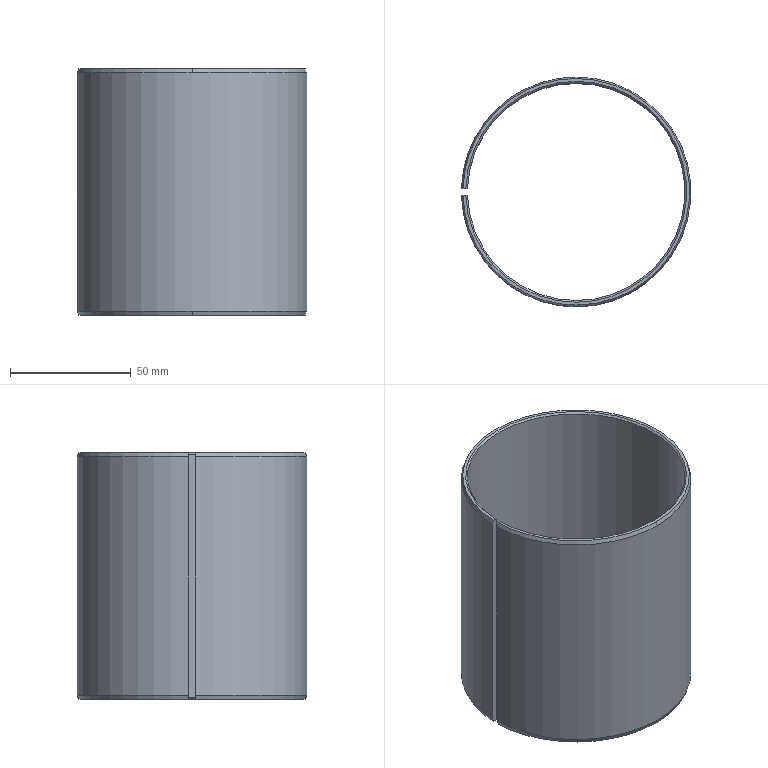Part | SolidWorks | features BaseBody 1 | 1 solid | 18 faces | box 94.981 x 95 x 102 mm | volume 72973 mm3 | cone 12 | plane 4 | cylinder 2 | commonest cylinder face diameters 90 x1 95 x1
STEP:
#1=CARTESIAN_POINT('',(1925.,-45.,-50.3));
#2=VERTEX_POINT('',#1);
#3=CARTESIAN_POINT('',(1880.02,-1.35,-50.3));
#4=VERTEX_POINT('',#3);
#5=CARTESIAN_POINT('',(1925.,0.,-50.3));
#6=DIRECTION('',(0.,0.,-1.));
#7=DIRECTION('',(-1.,0.,0.));
#8=AXIS2_PLACEMENT_3D('',#5,#6,#7);
#9=CIRCLE('',#8,45.);
#10=EDGE_CURVE('',#2,#4,#9,.T.);
#11=ORIENTED_EDGE('',*,*,#10,.F.);
#12=CARTESIAN_POINT('',(1925.,-45.7,-51.));
#13=VERTEX_POINT('',#12);
#14=CARTESIAN_POINT('',(1925.,-45.35,-50.65));
#15=DIRECTION('',(0.,-0.7071,-0.7071));
#16=VECTOR('',#15,1000.);
#17=LINE('',#14,#16);
#18=EDGE_CURVE('',#2,#13,#17,.T.);
#19=ORIENTED_EDGE('',*,*,#18,.T.);
#20=CARTESIAN_POINT('',(1879.32,-1.35,-51.));
#21=VERTEX_POINT('',#20);
#22=CARTESIAN_POINT('',(1925.,0.,-51.));
#23=DIRECTION('',(0.,0.,1.));
#24=DIRECTION('',(0.,1.,0.));
#25=AXIS2_PLACEMENT_3D('',#22,#23,#24);
#26=CIRCLE('',#25,45.7);
#27=EDGE_CURVE('',#21,#13,#26,.T.);
#28=ORIENTED_EDGE('',*,*,#27,.F.);
#29=CARTESIAN_POINT('',(1879.32,-1.35,-51.));
#30=CARTESIAN_POINT('',(1879.673,-1.35,-50.647));
#31=CARTESIAN_POINT('',(1880.02,-1.35,-50.3));
#32=B_SPLINE_CURVE_WITH_KNOTS('',2,(#29,#30,#31),.UNSPECIFIED.,.F.,.F.,(3,3),(0.,0.9902),.UNSPECIFIED.);
#33=EDGE_CURVE('',#21,#4,#32,.T.);
#34=ORIENTED_EDGE('',*,*,#33,.T.);
#35=EDGE_LOOP('',(#11,#19,#28,#34));
#36=FACE_OUTER_BOUND('',#35,.T.);
#37=CARTESIAN_POINT('',(1925.,0.,-50.65));
#38=DIRECTION('',(0.,0.,-1.));
#39=DIRECTION('',(0.,1.,0.));
#40=AXIS2_PLACEMENT_3D('',#37,#38,#39);
#41=CONICAL_SURFACE('',#40,45.35,0.7854);
#42=ADVANCED_FACE('',(#36),#41,.F.);
#43=ORIENTED_EDGE('',*,*,#18,.F.);
#44=CARTESIAN_POINT('',(1925.,45.,-50.3));
#45=VERTEX_POINT('',#44);
#46=CARTESIAN_POINT('',(1925.,0.,-50.3));
#47=DIRECTION('',(0.,0.,-1.));
#48=DIRECTION('',(-1.,0.,0.));
#49=AXIS2_PLACEMENT_3D('',#46,#47,#48);
#50=CIRCLE('',#49,45.);
#51=EDGE_CURVE('',#45,#2,#50,.T.);
#52=ORIENTED_EDGE('',*,*,#51,.F.);
#53=CARTESIAN_POINT('',(1925.,45.7,-51.));
#54=VERTEX_POINT('',#53);
#55=CARTESIAN_POINT('',(1925.,45.35,-50.65));
#56=DIRECTION('',(0.,0.7071,-0.7071));
#57=VECTOR('',#56,1000.);
#58=LINE('',#55,#57);
#59=EDGE_CURVE('',#45,#54,#58,.T.);
#60=ORIENTED_EDGE('',*,*,#59,.T.);
#61=CARTESIAN_POINT('',(1925.,0.,-51.));
#62=DIRECTION('',(0.,0.,1.));
#63=DIRECTION('',(0.,1.,0.));
#64=AXIS2_PLACEMENT_3D('',#61,#62,#63);
#65=CIRCLE('',#64,45.7);
#66=EDGE_CURVE('',#13,#54,#65,.T.);
#67=ORIENTED_EDGE('',*,*,#66,.F.);
#68=EDGE_LOOP('',(#43,#52,#60,#67));
#69=FACE_OUTER_BOUND('',#68,.T.);
#70=CARTESIAN_POINT('',(1925.,0.,-50.65));
#71=DIRECTION('',(0.,0.,-1.));
#72=DIRECTION('',(0.,1.,0.));
#73=AXIS2_PLACEMENT_3D('',#70,#71,#72);
#74=CONICAL_SURFACE('',#73,45.35,0.7854);
#75=ADVANCED_FACE('',(#69),#74,.F.);
#76=CARTESIAN_POINT('',(1925.,45.,50.3));
#77=VERTEX_POINT('',#76);
#78=CARTESIAN_POINT('',(1880.02,1.35,50.3));
#79=VERTEX_POINT('',#78);
#80=CARTESIAN_POINT('',(1925.,0.,50.3));
#81=DIRECTION('',(0.,0.,1.));
#82=DIRECTION('',(-1.,0.,0.));
#83=AXIS2_PLACEMENT_3D('',#80,#81,#82);
#84=CIRCLE('',#83,45.);
#85=EDGE_CURVE('',#77,#79,#84,.T.);
#86=ORIENTED_EDGE('',*,*,#85,.F.);
#87=CARTESIAN_POINT('',(1925.,45.7,51.));
#88=VERTEX_POINT('',#87);
#89=CARTESIAN_POINT('',(1925.,45.35,50.65));
#90=DIRECTION('',(0.,0.7071,0.7071));
#91=VECTOR('',#90,1000.);
#92=LINE('',#89,#91);
#93=EDGE_CURVE('',#77,#88,#92,.T.);
#94=ORIENTED_EDGE('',*,*,#93,.T.);
#95=CARTESIAN_POINT('',(1879.32,1.35,51.));
#96=VERTEX_POINT('',#95);
#97=CARTESIAN_POINT('',(1925.,0.,51.));
#98=DIRECTION('',(0.,0.,-1.));
#99=DIRECTION('',(0.,-1.,0.));
#100=AXIS2_PLACEMENT_3D('',#97,#98,#99);
#101=CIRCLE('',#100,45.7);
#102=EDGE_CURVE('',#96,#88,#101,.T.);
#103=ORIENTED_EDGE('',*,*,#102,.F.);
#104=CARTESIAN_POINT('',(1879.32,1.35,51.));
#105=CARTESIAN_POINT('',(1879.673,1.35,50.647));
#106=CARTESIAN_POINT('',(1880.02,1.35,50.3));
#107=B_SPLINE_CURVE_WITH_KNOTS('',2,(#104,#105,#106),.UNSPECIFIED.,.F.,.F.,(3,3),(0.,0.9902),.UNSPECIFIED.);
#108=EDGE_CURVE('',#96,#79,#107,.T.);
#109=ORIENTED_EDGE('',*,*,#108,.T.);
#110=EDGE_LOOP('',(#86,#94,#103,#109));
#111=FACE_OUTER_BOUND('',#110,.T.);
#112=CARTESIAN_POINT('',(1925.,0.,50.65));
#113=DIRECTION('',(0.,0.,1.));
#114=DIRECTION('',(0.,-1.,0.));
#115=AXIS2_PLACEMENT_3D('',#112,#113,#114);
#116=CONICAL_SURFACE('',#115,45.35,0.7854);
#117=ADVANCED_FACE('',(#111),#116,.F.);
#118=ORIENTED_EDGE('',*,*,#93,.F.);
#119=CARTESIAN_POINT('',(1925.,-45.,50.3));
#120=VERTEX_POINT('',#119);
#121=CARTESIAN_POINT('',(1925.,0.,50.3));
#122=DIRECTION('',(0.,0.,1.));
#123=DIRECTION('',(-1.,0.,0.));
#124=AXIS2_PLACEMENT_3D('',#121,#122,#123);
#125=CIRCLE('',#124,45.);
#126=EDGE_CURVE('',#120,#77,#125,.T.);
#127=ORIENTED_EDGE('',*,*,#126,.F.);
#128=CARTESIAN_POINT('',(1925.,-45.7,51.));
#129=VERTEX_POINT('',#128);
#130=CARTESIAN_POINT('',(1925.,-45.35,50.65));
#131=DIRECTION('',(0.,-0.7071,0.7071));
#132=VECTOR('',#131,1000.);
#133=LINE('',#130,#132);
#134=EDGE_CURVE('',#120,#129,#133,.T.);
#135=ORIENTED_EDGE('',*,*,#134,.T.);
#136=CARTESIAN_POINT('',(1925.,0.,51.));
#137=DIRECTION('',(0.,0.,-1.));
#138=DIRECTION('',(0.,-1.,0.));
#139=AXIS2_PLACEMENT_3D('',#136,#137,#138);
#140=CIRCLE('',#139,45.7);
#141=EDGE_CURVE('',#88,#129,#140,.T.);
#142=ORIENTED_EDGE('',*,*,#141,.F.);
#143=EDGE_LOOP('',(#118,#127,#135,#142));
#144=FACE_OUTER_BOUND('',#143,.T.);
#145=CARTESIAN_POINT('',(1925.,0.,50.65));
#146=DIRECTION('',(0.,0.,1.));
#147=DIRECTION('',(0.,-1.,0.));
#148=AXIS2_PLACEMENT_3D('',#145,#146,#147);
#149=CONICAL_SURFACE('',#148,45.35,0.7854);
#150=ADVANCED_FACE('',(#144),#149,.F.);
#151=CARTESIAN_POINT('',(1925.,46.888,-51.));
#152=VERTEX_POINT('',#151);
#153=CARTESIAN_POINT('',(1925.,-46.888,-51.));
#154=VERTEX_POINT('',#153);
#155=CARTESIAN_POINT('',(1925.,0.,-51.));
#156=DIRECTION('',(0.,0.,-1.));
#157=DIRECTION('',(0.,-1.,0.));
#158=AXIS2_PLACEMENT_3D('',#155,#156,#157);
#159=CIRCLE('',#158,46.888);
#160=EDGE_CURVE('',#152,#154,#159,.T.);
#161=ORIENTED_EDGE('',*,*,#160,.F.);
#162=CARTESIAN_POINT('',(1925.,47.5,-49.319));
#163=VERTEX_POINT('',#162);
#164=CARTESIAN_POINT('',(1925.,47.194,-50.159));
#165=DIRECTION('',(0.,0.342,0.9397));
#166=VECTOR('',#165,1000.);
#167=LINE('',#164,#166);
#168=EDGE_CURVE('',#152,#163,#167,.T.);
#169=ORIENTED_EDGE('',*,*,#168,.T.);
#170=CARTESIAN_POINT('',(1925.,-47.5,-49.319));
#171=VERTEX_POINT('',#170);
#172=CARTESIAN_POINT('',(1925.,0.,-49.319));
#173=DIRECTION('',(0.,0.,1.));
#174=DIRECTION('',(-1.,0.,0.));
#175=AXIS2_PLACEMENT_3D('',#172,#173,#174);
#176=CIRCLE('',#175,47.5);
#177=EDGE_CURVE('',#171,#163,#176,.T.);
#178=ORIENTED_EDGE('',*,*,#177,.F.);
#179=CARTESIAN_POINT('',(1925.,-47.194,-50.159));
#180=DIRECTION('',(0.,-0.342,0.9397));
#181=VECTOR('',#180,1000.);
#182=LINE('',#179,#181);
#183=EDGE_CURVE('',#154,#171,#182,.T.);
#184=ORIENTED_EDGE('',*,*,#183,.F.);
#185=EDGE_LOOP('',(#161,#169,#178,#184));
#186=FACE_OUTER_BOUND('',#185,.T.);
#187=CARTESIAN_POINT('',(1925.,0.,-50.159));
#188=DIRECTION('',(0.,0.,1.));
#189=DIRECTION('',(0.,-1.,0.));
#190=AXIS2_PLACEMENT_3D('',#187,#188,#189);
#191=CONICAL_SURFACE('',#190,47.194,0.3491);
#192=ADVANCED_FACE('',(#186),#191,.T.);
#193=CARTESIAN_POINT('',(1878.131,-1.35,-51.));
#194=VERTEX_POINT('',#193);
#195=CARTESIAN_POINT('',(1925.,0.,-51.));
#196=DIRECTION('',(0.,0.,-1.));
#197=DIRECTION('',(0.,-1.,0.));
#198=AXIS2_PLACEMENT_3D('',#195,#196,#197);
#199=CIRCLE('',#198,46.888);
#200=EDGE_CURVE('',#154,#194,#199,.T.);
#201=ORIENTED_EDGE('',*,*,#200,.F.);
#202=ORIENTED_EDGE('',*,*,#183,.T.);
#203=CARTESIAN_POINT('',(1877.519,-1.35,-49.319));
#204=VERTEX_POINT('',#203);
#205=CARTESIAN_POINT('',(1925.,0.,-49.319));
#206=DIRECTION('',(0.,0.,1.));
#207=DIRECTION('',(-1.,0.,0.));
#208=AXIS2_PLACEMENT_3D('',#205,#206,#207);
#209=CIRCLE('',#208,47.5);
#210=EDGE_CURVE('',#204,#171,#209,.T.);
#211=ORIENTED_EDGE('',*,*,#210,.F.);
#212=CARTESIAN_POINT('',(1877.519,-1.35,-49.319));
#213=CARTESIAN_POINT('',(1877.827,-1.35,-50.165));
#214=CARTESIAN_POINT('',(1878.131,-1.35,-51.));
#215=B_SPLINE_CURVE_WITH_KNOTS('',2,(#212,#213,#214),.UNSPECIFIED.,.F.,.F.,(3,3),(0.,1.789),.UNSPECIFIED.);
#216=EDGE_CURVE('',#204,#194,#215,.T.);
#217=ORIENTED_EDGE('',*,*,#216,.T.);
#218=EDGE_LOOP('',(#201,#202,#211,#217));
#219=FACE_OUTER_BOUND('',#218,.T.);
#220=CARTESIAN_POINT('',(1925.,0.,-50.159));
#221=DIRECTION('',(0.,0.,1.));
#222=DIRECTION('',(0.,-1.,0.));
#223=AXIS2_PLACEMENT_3D('',#220,#221,#222);
#224=CONICAL_SURFACE('',#223,47.194,0.3491);
#225=ADVANCED_FACE('',(#219),#224,.T.);
#226=CARTESIAN_POINT('',(1925.,-46.888,51.));
#227=VERTEX_POINT('',#226);
#228=CARTESIAN_POINT('',(1925.,46.888,51.));
#229=VERTEX_POINT('',#228);
#230=CARTESIAN_POINT('',(1925.,0.,51.));
#231=DIRECTION('',(0.,0.,1.));
#232=DIRECTION('',(0.,1.,0.));
#233=AXIS2_PLACEMENT_3D('',#230,#231,#232);
#234=CIRCLE('',#233,46.888);
#235=EDGE_CURVE('',#227,#229,#234,.T.);
#236=ORIENTED_EDGE('',*,*,#235,.F.);
#237=CARTESIAN_POINT('',(1925.,-47.5,49.319));
#238=VERTEX_POINT('',#237);
#239=CARTESIAN_POINT('',(1925.,-47.194,50.159));
#240=DIRECTION('',(0.,-0.342,-0.9397));
#241=VECTOR('',#240,1000.);
#242=LINE('',#239,#241);
#243=EDGE_CURVE('',#227,#238,#242,.T.);
#244=ORIENTED_EDGE('',*,*,#243,.T.);
#245=CARTESIAN_POINT('',(1925.,47.5,49.319));
#246=VERTEX_POINT('',#245);
#247=CARTESIAN_POINT('',(1925.,0.,49.319));
#248=DIRECTION('',(0.,0.,-1.));
#249=DIRECTION('',(-1.,0.,0.));
#250=AXIS2_PLACEMENT_3D('',#247,#248,#249);
#251=CIRCLE('',#250,47.5);
#252=EDGE_CURVE('',#246,#238,#251,.T.);
#253=ORIENTED_EDGE('',*,*,#252,.F.);
#254=CARTESIAN_POINT('',(1925.,47.194,50.159));
#255=DIRECTION('',(0.,0.342,-0.9397));
#256=VECTOR('',#255,1000.);
#257=LINE('',#254,#256);
#258=EDGE_CURVE('',#229,#246,#257,.T.);
#259=ORIENTED_EDGE('',*,*,#258,.F.);
#260=EDGE_LOOP('',(#236,#244,#253,#259));
#261=FACE_OUTER_BOUND('',#260,.T.);
#262=CARTESIAN_POINT('',(1925.,0.,50.159));
#263=DIRECTION('',(0.,0.,-1.));
#264=DIRECTION('',(0.,1.,0.));
#265=AXIS2_PLACEMENT_3D('',#262,#263,#264);
#266=CONICAL_SURFACE('',#265,47.194,0.3491);
#267=ADVANCED_FACE('',(#261),#266,.T.);
#268=CARTESIAN_POINT('',(1878.131,1.35,51.));
#269=VERTEX_POINT('',#268);
#270=CARTESIAN_POINT('',(1925.,0.,51.));
#271=DIRECTION('',(0.,0.,1.));
#272=DIRECTION('',(0.,1.,0.));
#273=AXIS2_PLACEMENT_3D('',#270,#271,#272);
#274=CIRCLE('',#273,46.888);
#275=EDGE_CURVE('',#229,#269,#274,.T.);
#276=ORIENTED_EDGE('',*,*,#275,.F.);
#277=ORIENTED_EDGE('',*,*,#258,.T.);
#278=CARTESIAN_POINT('',(1877.519,1.35,49.319));
#279=VERTEX_POINT('',#278);
#280=CARTESIAN_POINT('',(1925.,0.,49.319));
#281=DIRECTION('',(0.,0.,-1.));
#282=DIRECTION('',(-1.,0.,0.));
#283=AXIS2_PLACEMENT_3D('',#280,#281,#282);
#284=CIRCLE('',#283,47.5);
#285=EDGE_CURVE('',#279,#246,#284,.T.);
#286=ORIENTED_EDGE('',*,*,#285,.F.);
#287=CARTESIAN_POINT('',(1877.519,1.35,49.319));
#288=CARTESIAN_POINT('',(1877.827,1.35,50.165));
#289=CARTESIAN_POINT('',(1878.131,1.35,51.));
#290=B_SPLINE_CURVE_WITH_KNOTS('',2,(#287,#288,#289),.UNSPECIFIED.,.F.,.F.,(3,3),(0.,1.789),.UNSPECIFIED.);
#291=EDGE_CURVE('',#279,#269,#290,.T.);
#292=ORIENTED_EDGE('',*,*,#291,.T.);
#293=EDGE_LOOP('',(#276,#277,#286,#292));
#294=FACE_OUTER_BOUND('',#293,.T.);
#295=CARTESIAN_POINT('',(1925.,0.,50.159));
#296=DIRECTION('',(0.,0.,-1.));
#297=DIRECTION('',(0.,1.,0.));
#298=AXIS2_PLACEMENT_3D('',#295,#296,#297);
#299=CONICAL_SURFACE('',#298,47.194,0.3491);
#300=ADVANCED_FACE('',(#294),#299,.T.);
#301=CARTESIAN_POINT('',(1902.5,-1.35,-51.));
#302=DIRECTION('',(1.,0.,0.));
#303=VECTOR('',#302,1000.);
#304=LINE('',#301,#303);
#305=EDGE_CURVE('',#194,#21,#304,.T.);
#306=ORIENTED_EDGE('',*,*,#305,.T.);
#307=ORIENTED_EDGE('',*,*,#27,.T.);
#308=ORIENTED_EDGE('',*,*,#66,.T.);
#309=CARTESIAN_POINT('',(1879.32,1.35,-51.));
#310=VERTEX_POINT('',#309);
#311=CARTESIAN_POINT('',(1925.,0.,-51.));
#312=DIRECTION('',(0.,0.,1.));
#313=DIRECTION('',(0.,1.,0.));
#314=AXIS2_PLACEMENT_3D('',#311,#312,#313);
#315=CIRCLE('',#314,45.7);
#316=EDGE_CURVE('',#54,#310,#315,.T.);
#317=ORIENTED_EDGE('',*,*,#316,.T.);
#318=CARTESIAN_POINT('',(1878.131,1.35,-51.));
#319=VERTEX_POINT('',#318);
#320=CARTESIAN_POINT('',(1902.5,1.35,-51.));
#321=DIRECTION('',(-1.,0.,0.));
#322=VECTOR('',#321,1000.);
#323=LINE('',#320,#322);
#324=EDGE_CURVE('',#310,#319,#323,.T.);
#325=ORIENTED_EDGE('',*,*,#324,.T.);
#326=CARTESIAN_POINT('',(1925.,0.,-51.));
#327=DIRECTION('',(0.,0.,-1.));
#328=DIRECTION('',(0.,-1.,0.));
#329=AXIS2_PLACEMENT_3D('',#326,#327,#328);
#330=CIRCLE('',#329,46.888);
#331=EDGE_CURVE('',#319,#152,#330,.T.);
#332=ORIENTED_EDGE('',*,*,#331,.T.);
#333=ORIENTED_EDGE('',*,*,#160,.T.);
#334=ORIENTED_EDGE('',*,*,#200,.T.);
#335=EDGE_LOOP('',(#306,#307,#308,#317,#325,#332,#333,#334));
#336=FACE_OUTER_BOUND('',#335,.T.);
#337=CARTESIAN_POINT('',(1925.,0.,-51.));
#338=DIRECTION('',(0.,0.,-1.));
#339=DIRECTION('',(-1.,0.,0.));
#340=AXIS2_PLACEMENT_3D('',#337,#338,#339);
#341=PLANE('',#340);
#342=ADVANCED_FACE('',(#336),#341,.T.);
#343=CARTESIAN_POINT('',(1877.519,-1.35,49.319));
#344=VERTEX_POINT('',#343);
#345=CARTESIAN_POINT('',(1877.519,-1.35,0.));
#346=DIRECTION('',(0.,0.,-1.));
#347=VECTOR('',#346,1000.);
#348=LINE('',#345,#347);
#349=EDGE_CURVE('',#344,#204,#348,.T.);
#350=ORIENTED_EDGE('',*,*,#349,.T.);
#351=ORIENTED_EDGE('',*,*,#210,.T.);
#352=ORIENTED_EDGE('',*,*,#177,.T.);
#353=CARTESIAN_POINT('',(1877.519,1.35,-49.319));
#354=VERTEX_POINT('',#353);
#355=CARTESIAN_POINT('',(1925.,0.,-49.319));
#356=DIRECTION('',(0.,0.,1.));
#357=DIRECTION('',(-1.,0.,0.));
#358=AXIS2_PLACEMENT_3D('',#355,#356,#357);
#359=CIRCLE('',#358,47.5);
#360=EDGE_CURVE('',#163,#354,#359,.T.);
#361=ORIENTED_EDGE('',*,*,#360,.T.);
#362=CARTESIAN_POINT('',(1877.519,1.35,0.));
#363=DIRECTION('',(0.,0.,1.));
#364=VECTOR('',#363,1000.);
#365=LINE('',#362,#364);
#366=EDGE_CURVE('',#354,#279,#365,.T.);
#367=ORIENTED_EDGE('',*,*,#366,.T.);
#368=ORIENTED_EDGE('',*,*,#285,.T.);
#369=ORIENTED_EDGE('',*,*,#252,.T.);
#370=CARTESIAN_POINT('',(1925.,0.,49.319));
#371=DIRECTION('',(0.,0.,-1.));
#372=DIRECTION('',(-1.,0.,0.));
#373=AXIS2_PLACEMENT_3D('',#370,#371,#372);
#374=CIRCLE('',#373,47.5);
#375=EDGE_CURVE('',#238,#344,#374,.T.);
#376=ORIENTED_EDGE('',*,*,#375,.T.);
#377=EDGE_LOOP('',(#350,#351,#352,#361,#367,#368,#369,#376));
#378=FACE_OUTER_BOUND('',#377,.T.);
#379=CARTESIAN_POINT('',(1925.,0.,0.));
#380=DIRECTION('',(0.,0.,1.));
#381=DIRECTION('',(-1.,0.,0.));
#382=AXIS2_PLACEMENT_3D('',#379,#380,#381);
#383=CYLINDRICAL_SURFACE('',#382,47.5);
#384=ADVANCED_FACE('',(#378),#383,.T.);
#385=ORIENTED_EDGE('',*,*,#243,.F.);
#386=CARTESIAN_POINT('',(1878.131,-1.35,51.));
#387=VERTEX_POINT('',#386);
#388=CARTESIAN_POINT('',(1925.,0.,51.));
#389=DIRECTION('',(0.,0.,1.));
#390=DIRECTION('',(0.,1.,0.));
#391=AXIS2_PLACEMENT_3D('',#388,#389,#390);
#392=CIRCLE('',#391,46.888);
#393=EDGE_CURVE('',#387,#227,#392,.T.);
#394=ORIENTED_EDGE('',*,*,#393,.F.);
#395=CARTESIAN_POINT('',(1878.131,-1.35,51.));
#396=CARTESIAN_POINT('',(1877.827,-1.35,50.165));
#397=CARTESIAN_POINT('',(1877.519,-1.35,49.319));
#398=B_SPLINE_CURVE_WITH_KNOTS('',2,(#395,#396,#397),.UNSPECIFIED.,.F.,.F.,(3,3),(0.,1.789),.UNSPECIFIED.);
#399=EDGE_CURVE('',#387,#344,#398,.T.);
#400=ORIENTED_EDGE('',*,*,#399,.T.);
#401=ORIENTED_EDGE('',*,*,#375,.F.);
#402=EDGE_LOOP('',(#385,#394,#400,#401));
#403=FACE_OUTER_BOUND('',#402,.T.);
#404=CARTESIAN_POINT('',(1925.,0.,50.159));
#405=DIRECTION('',(0.,0.,-1.));
#406=DIRECTION('',(0.,1.,0.));
#407=AXIS2_PLACEMENT_3D('',#404,#405,#406);
#408=CONICAL_SURFACE('',#407,47.194,0.3491);
#409=ADVANCED_FACE('',(#403),#408,.T.);
#410=ORIENTED_EDGE('',*,*,#168,.F.);
#411=ORIENTED_EDGE('',*,*,#331,.F.);
#412=CARTESIAN_POINT('',(1878.131,1.35,-51.));
#413=CARTESIAN_POINT('',(1877.827,1.35,-50.165));
#414=CARTESIAN_POINT('',(1877.519,1.35,-49.319));
#415=B_SPLINE_CURVE_WITH_KNOTS('',2,(#412,#413,#414),.UNSPECIFIED.,.F.,.F.,(3,3),(0.,1.789),.UNSPECIFIED.);
#416=EDGE_CURVE('',#319,#354,#415,.T.);
#417=ORIENTED_EDGE('',*,*,#416,.T.);
#418=ORIENTED_EDGE('',*,*,#360,.F.);
#419=EDGE_LOOP('',(#410,#411,#417,#418));
#420=FACE_OUTER_BOUND('',#419,.T.);
#421=CARTESIAN_POINT('',(1925.,0.,-50.159));
#422=DIRECTION('',(0.,0.,1.));
#423=DIRECTION('',(0.,-1.,0.));
#424=AXIS2_PLACEMENT_3D('',#421,#422,#423);
#425=CONICAL_SURFACE('',#424,47.194,0.3491);
#426=ADVANCED_FACE('',(#420),#425,.T.);
#427=CARTESIAN_POINT('',(1879.32,-1.35,51.));
#428=VERTEX_POINT('',#427);
#429=CARTESIAN_POINT('',(1902.5,-1.35,51.));
#430=DIRECTION('',(-1.,0.,0.));
#431=VECTOR('',#430,1000.);
#432=LINE('',#429,#431);
#433=EDGE_CURVE('',#428,#387,#432,.T.);
#434=ORIENTED_EDGE('',*,*,#433,.T.);
#435=ORIENTED_EDGE('',*,*,#393,.T.);
#436=ORIENTED_EDGE('',*,*,#235,.T.);
#437=ORIENTED_EDGE('',*,*,#275,.T.);
#438=CARTESIAN_POINT('',(1902.5,1.35,51.));
#439=DIRECTION('',(1.,0.,0.));
#440=VECTOR('',#439,1000.);
#441=LINE('',#438,#440);
#442=EDGE_CURVE('',#269,#96,#441,.T.);
#443=ORIENTED_EDGE('',*,*,#442,.T.);
#444=ORIENTED_EDGE('',*,*,#102,.T.);
#445=ORIENTED_EDGE('',*,*,#141,.T.);
#446=CARTESIAN_POINT('',(1925.,0.,51.));
#447=DIRECTION('',(0.,0.,-1.));
#448=DIRECTION('',(0.,-1.,0.));
#449=AXIS2_PLACEMENT_3D('',#446,#447,#448);
#450=CIRCLE('',#449,45.7);
#451=EDGE_CURVE('',#129,#428,#450,.T.);
#452=ORIENTED_EDGE('',*,*,#451,.T.);
#453=EDGE_LOOP('',(#434,#435,#436,#437,#443,#444,#445,#452));
#454=FACE_OUTER_BOUND('',#453,.T.);
#455=CARTESIAN_POINT('',(1925.,0.,51.));
#456=DIRECTION('',(0.,0.,1.));
#457=DIRECTION('',(1.,0.,0.));
#458=AXIS2_PLACEMENT_3D('',#455,#456,#457);
#459=PLANE('',#458);
#460=ADVANCED_FACE('',(#454),#459,.T.);
#461=ORIENTED_EDGE('',*,*,#134,.F.);
#462=CARTESIAN_POINT('',(1880.02,-1.35,50.3));
#463=VERTEX_POINT('',#462);
#464=CARTESIAN_POINT('',(1925.,0.,50.3));
#465=DIRECTION('',(0.,0.,1.));
#466=DIRECTION('',(-1.,0.,0.));
#467=AXIS2_PLACEMENT_3D('',#464,#465,#466);
#468=CIRCLE('',#467,45.);
#469=EDGE_CURVE('',#463,#120,#468,.T.);
#470=ORIENTED_EDGE('',*,*,#469,.F.);
#471=CARTESIAN_POINT('',(1880.02,-1.35,50.3));
#472=CARTESIAN_POINT('',(1879.673,-1.35,50.647));
#473=CARTESIAN_POINT('',(1879.32,-1.35,51.));
#474=B_SPLINE_CURVE_WITH_KNOTS('',2,(#471,#472,#473),.UNSPECIFIED.,.F.,.F.,(3,3),(0.,0.9902),.UNSPECIFIED.);
#475=EDGE_CURVE('',#463,#428,#474,.T.);
#476=ORIENTED_EDGE('',*,*,#475,.T.);
#477=ORIENTED_EDGE('',*,*,#451,.F.);
#478=EDGE_LOOP('',(#461,#470,#476,#477));
#479=FACE_OUTER_BOUND('',#478,.T.);
#480=CARTESIAN_POINT('',(1925.,0.,50.65));
#481=DIRECTION('',(0.,0.,1.));
#482=DIRECTION('',(0.,-1.,0.));
#483=AXIS2_PLACEMENT_3D('',#480,#481,#482);
#484=CONICAL_SURFACE('',#483,45.35,0.7854);
#485=ADVANCED_FACE('',(#479),#484,.F.);
#486=ORIENTED_EDGE('',*,*,#59,.F.);
#487=CARTESIAN_POINT('',(1880.02,1.35,-50.3));
#488=VERTEX_POINT('',#487);
#489=CARTESIAN_POINT('',(1925.,0.,-50.3));
#490=DIRECTION('',(0.,0.,-1.));
#491=DIRECTION('',(-1.,0.,0.));
#492=AXIS2_PLACEMENT_3D('',#489,#490,#491);
#493=CIRCLE('',#492,45.);
#494=EDGE_CURVE('',#488,#45,#493,.T.);
#495=ORIENTED_EDGE('',*,*,#494,.F.);
#496=CARTESIAN_POINT('',(1880.02,1.35,-50.3));
#497=CARTESIAN_POINT('',(1879.673,1.35,-50.647));
#498=CARTESIAN_POINT('',(1879.32,1.35,-51.));
#499=B_SPLINE_CURVE_WITH_KNOTS('',2,(#496,#497,#498),.UNSPECIFIED.,.F.,.F.,(3,3),(0.,0.9902),.UNSPECIFIED.);
#500=EDGE_CURVE('',#488,#310,#499,.T.);
#501=ORIENTED_EDGE('',*,*,#500,.T.);
#502=ORIENTED_EDGE('',*,*,#316,.F.);
#503=EDGE_LOOP('',(#486,#495,#501,#502));
#504=FACE_OUTER_BOUND('',#503,.T.);
#505=CARTESIAN_POINT('',(1925.,0.,-50.65));
#506=DIRECTION('',(0.,0.,-1.));
#507=DIRECTION('',(0.,1.,0.));
#508=AXIS2_PLACEMENT_3D('',#505,#506,#507);
#509=CONICAL_SURFACE('',#508,45.35,0.7854);
#510=ADVANCED_FACE('',(#504),#509,.F.);
#511=CARTESIAN_POINT('',(1880.02,-1.35,0.));
#512=DIRECTION('',(0.,0.,1.));
#513=VECTOR('',#512,1000.);
#514=LINE('',#511,#513);
#515=EDGE_CURVE('',#4,#463,#514,.T.);
#516=ORIENTED_EDGE('',*,*,#515,.T.);
#517=ORIENTED_EDGE('',*,*,#469,.T.);
#518=ORIENTED_EDGE('',*,*,#126,.T.);
#519=ORIENTED_EDGE('',*,*,#85,.T.);
#520=CARTESIAN_POINT('',(1880.02,1.35,0.));
#521=DIRECTION('',(0.,0.,-1.));
#522=VECTOR('',#521,1000.);
#523=LINE('',#520,#522);
#524=EDGE_CURVE('',#79,#488,#523,.T.);
#525=ORIENTED_EDGE('',*,*,#524,.T.);
#526=ORIENTED_EDGE('',*,*,#494,.T.);
#527=ORIENTED_EDGE('',*,*,#51,.T.);
#528=ORIENTED_EDGE('',*,*,#10,.T.);
#529=EDGE_LOOP('',(#516,#517,#518,#519,#525,#526,#527,#528));
#530=FACE_OUTER_BOUND('',#529,.T.);
#531=CARTESIAN_POINT('',(1925.,0.,0.));
#532=DIRECTION('',(0.,0.,1.));
#533=DIRECTION('',(-1.,0.,0.));
#534=AXIS2_PLACEMENT_3D('',#531,#532,#533);
#535=CYLINDRICAL_SURFACE('',#534,45.);
#536=ADVANCED_FACE('',(#530),#535,.F.);
#537=ORIENTED_EDGE('',*,*,#291,.F.);
#538=ORIENTED_EDGE('',*,*,#366,.F.);
#539=ORIENTED_EDGE('',*,*,#416,.F.);
#540=ORIENTED_EDGE('',*,*,#324,.F.);
#541=ORIENTED_EDGE('',*,*,#500,.F.);
#542=ORIENTED_EDGE('',*,*,#524,.F.);
#543=ORIENTED_EDGE('',*,*,#108,.F.);
#544=ORIENTED_EDGE('',*,*,#442,.F.);
#545=EDGE_LOOP('',(#537,#538,#539,#540,#541,#542,#543,#544));
#546=FACE_OUTER_BOUND('',#545,.T.);
#547=CARTESIAN_POINT('',(1880.,1.35,0.));
#548=DIRECTION('',(0.,-1.,0.));
#549=DIRECTION('',(0.,0.,1.));
#550=AXIS2_PLACEMENT_3D('',#547,#548,#549);
#551=PLANE('',#550);
#552=ADVANCED_FACE('',(#546),#551,.T.);
#553=ORIENTED_EDGE('',*,*,#399,.F.);
#554=ORIENTED_EDGE('',*,*,#433,.F.);
#555=ORIENTED_EDGE('',*,*,#475,.F.);
#556=ORIENTED_EDGE('',*,*,#515,.F.);
#557=ORIENTED_EDGE('',*,*,#33,.F.);
#558=ORIENTED_EDGE('',*,*,#305,.F.);
#559=ORIENTED_EDGE('',*,*,#216,.F.);
#560=ORIENTED_EDGE('',*,*,#349,.F.);
#561=EDGE_LOOP('',(#553,#554,#555,#556,#557,#558,#559,#560));
#562=FACE_OUTER_BOUND('',#561,.T.);
#563=CARTESIAN_POINT('',(1880.,-1.35,0.));
#564=DIRECTION('',(0.,1.,0.));
#565=DIRECTION('',(0.,0.,-1.));
#566=AXIS2_PLACEMENT_3D('',#563,#564,#565);
#567=PLANE('',#566);
#568=ADVANCED_FACE('',(#562),#567,.T.);
#569=CLOSED_SHELL('',(#42,#75,#117,#150,#192,#225,#267,#300,#342,#384,#409,#426,#460,#485,#510,#536,#552,#568));
#570=MANIFOLD_SOLID_BREP('',#569);
#571=CARTESIAN_POINT('',(0.,0.,0.));
#572=DIRECTION('',(0.,0.,1.));
#573=DIRECTION('',(1.,0.,0.));
#574=AXIS2_PLACEMENT_3D('',#571,#572,#573);
#575=(LENGTH_UNIT()NAMED_UNIT(*)SI_UNIT(.MILLI.,.METRE.));
#576=UNCERTAINTY_MEASURE_WITH_UNIT(LENGTH_MEASURE(0.00001),#575,'','');
#577=(NAMED_UNIT(*)PLANE_ANGLE_UNIT()SI_UNIT($,.RADIAN.));
#578=(NAMED_UNIT(*)SI_UNIT($,.STERADIAN.)SOLID_ANGLE_UNIT());
#579=(GEOMETRIC_REPRESENTATION_CONTEXT(3)GLOBAL_UNCERTAINTY_ASSIGNED_CONTEXT((#576))GLOBAL_UNIT_ASSIGNED_CONTEXT((#575,#577,#578))REPRESENTATION_CONTEXT('',''));
#580=ADVANCED_BREP_SHAPE_REPRESENTATION('',(#570,#574),#579);